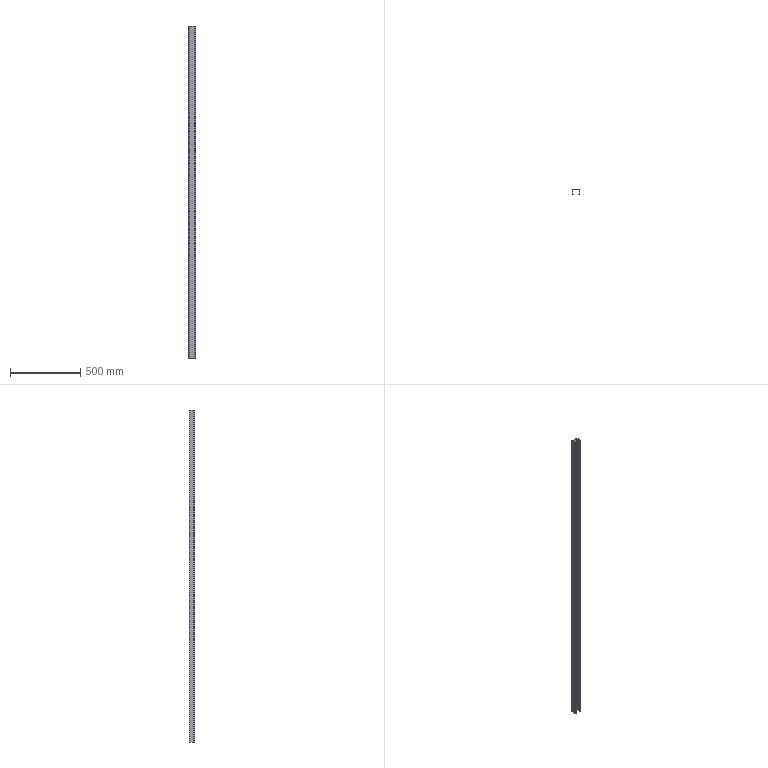Part | STEP file | 31E-01025QY25 | 1 solid | 28 faces | box 50 x 38.192 x 2366 mm | volume 389538 mm3 | plane 16 | cylinder 12 | commonest cylinder face diameters 1 x4 2 x4 4 x2 26 x2
STEP:
#1=CARTESIAN_POINT('',(27.993,8.298,1183.));
#2=VERTEX_POINT('',#1);
#3=CARTESIAN_POINT('',(32.281,3.187,1183.));
#4=VERTEX_POINT('',#3);
#5=CARTESIAN_POINT('',(30.137,5.743,1183.));
#6=DIRECTION('',(0.6428,-0.766,0.));
#7=VECTOR('',#6,1.);
#8=LINE('',#5,#7);
#9=EDGE_CURVE('',#2,#4,#8,.T.);
#10=ORIENTED_EDGE('',*,*,#9,.F.);
#11=CARTESIAN_POINT('',(27.993,8.298,-1183.));
#12=VERTEX_POINT('',#11);
#13=CARTESIAN_POINT('',(27.993,8.298,0.));
#14=DIRECTION('',(0.,0.,-1.));
#15=VECTOR('',#14,1.);
#16=LINE('',#13,#15);
#17=EDGE_CURVE('',#2,#12,#16,.T.);
#18=ORIENTED_EDGE('',*,*,#17,.T.);
#19=CARTESIAN_POINT('',(32.281,3.187,-1183.));
#20=VERTEX_POINT('',#19);
#21=CARTESIAN_POINT('',(30.137,5.743,-1183.));
#22=DIRECTION('',(0.6428,-0.766,0.));
#23=VECTOR('',#22,1.);
#24=LINE('',#21,#23);
#25=EDGE_CURVE('',#12,#20,#24,.T.);
#26=ORIENTED_EDGE('',*,*,#25,.T.);
#27=CARTESIAN_POINT('',(32.281,3.187,0.));
#28=DIRECTION('',(0.,0.,-1.));
#29=VECTOR('',#28,1.);
#30=LINE('',#27,#29);
#31=EDGE_CURVE('',#4,#20,#30,.T.);
#32=ORIENTED_EDGE('',*,*,#31,.F.);
#33=EDGE_LOOP('',(#10,#18,#26,#32));
#34=FACE_OUTER_BOUND('',#33,.T.);
#35=CARTESIAN_POINT('',(27.525,8.856,1183.));
#36=DIRECTION('',(0.766,0.6428,0.));
#37=DIRECTION('',(-0.6428,0.766,0.));
#38=AXIS2_PLACEMENT_3D('',#35,#36,#37);
#39=PLANE('',#38);
#40=ADVANCED_FACE('',(#34),#39,.F.);
#41=CARTESIAN_POINT('',(76.525,38.856,1183.));
#42=VERTEX_POINT('',#41);
#43=CARTESIAN_POINT('',(28.525,38.856,1183.));
#44=VERTEX_POINT('',#43);
#45=CARTESIAN_POINT('',(52.525,38.856,1183.));
#46=DIRECTION('',(-1.,0.,0.));
#47=VECTOR('',#46,1.);
#48=LINE('',#45,#47);
#49=EDGE_CURVE('',#42,#44,#48,.T.);
#50=ORIENTED_EDGE('',*,*,#49,.T.);
#51=CARTESIAN_POINT('',(27.525,37.856,1183.));
#52=VERTEX_POINT('',#51);
#53=CARTESIAN_POINT('',(28.525,37.856,1183.));
#54=DIRECTION('',(0.,0.,1.));
#55=AXIS2_PLACEMENT_3D('',#53,#54,$);
#56=CIRCLE('',#55,1.);
#57=EDGE_CURVE('',#44,#52,#56,.T.);
#58=ORIENTED_EDGE('',*,*,#57,.T.);
#59=CARTESIAN_POINT('',(27.525,9.584,1183.));
#60=VERTEX_POINT('',#59);
#61=CARTESIAN_POINT('',(27.525,23.72,1183.));
#62=DIRECTION('',(0.,-1.,0.));
#63=VECTOR('',#62,1.);
#64=LINE('',#61,#63);
#65=EDGE_CURVE('',#52,#60,#64,.T.);
#66=ORIENTED_EDGE('',*,*,#65,.T.);
#67=CARTESIAN_POINT('',(29.525,9.584,1183.));
#68=DIRECTION('',(0.,0.,1.));
#69=AXIS2_PLACEMENT_3D('',#67,#68,$);
#70=CIRCLE('',#69,2.);
#71=EDGE_CURVE('',#60,#2,#70,.T.);
#72=ORIENTED_EDGE('',*,*,#71,.T.);
#73=ORIENTED_EDGE('',*,*,#9,.T.);
#74=CARTESIAN_POINT('',(28.342,2.493,1183.));
#75=VERTEX_POINT('',#74);
#76=CARTESIAN_POINT('',(30.312,2.84,1183.));
#77=DIRECTION('',(-0.9848,-0.1736,0.));
#78=VECTOR('',#77,1.);
#79=LINE('',#76,#78);
#80=EDGE_CURVE('',#4,#75,#79,.T.);
#81=ORIENTED_EDGE('',*,*,#80,.T.);
#82=CARTESIAN_POINT('',(32.653,0.6877,1183.));
#83=VERTEX_POINT('',#82);
#84=CARTESIAN_POINT('',(35.437,13.386,1183.));
#85=DIRECTION('',(0.,0.,1.));
#86=AXIS2_PLACEMENT_3D('',#84,#85,$);
#87=CIRCLE('',#86,13.);
#88=EDGE_CURVE('',#75,#83,#87,.T.);
#89=ORIENTED_EDGE('',*,*,#88,.T.);
#90=CARTESIAN_POINT('',(33.867,1.665,1183.));
#91=VERTEX_POINT('',#90);
#92=CARTESIAN_POINT('',(32.867,1.665,1183.));
#93=DIRECTION('',(0.,0.,1.));
#94=AXIS2_PLACEMENT_3D('',#92,#93,$);
#95=CIRCLE('',#94,1.);
#96=EDGE_CURVE('',#83,#91,#95,.T.);
#97=ORIENTED_EDGE('',*,*,#96,.T.);
#98=CARTESIAN_POINT('',(33.867,2.983,1183.));
#99=VERTEX_POINT('',#98);
#100=CARTESIAN_POINT('',(33.867,2.324,1183.));
#101=DIRECTION('',(0.,1.,0.));
#102=VECTOR('',#101,1.);
#103=LINE('',#100,#102);
#104=EDGE_CURVE('',#91,#99,#103,.T.);
#105=ORIENTED_EDGE('',*,*,#104,.T.);
#106=CARTESIAN_POINT('',(33.75,3.304,1183.));
#107=VERTEX_POINT('',#106);
#108=CARTESIAN_POINT('',(33.367,2.983,1183.));
#109=DIRECTION('',(0.,0.,1.));
#110=AXIS2_PLACEMENT_3D('',#108,#109,$);
#111=CIRCLE('',#110,0.5);
#112=EDGE_CURVE('',#99,#107,#111,.T.);
#113=ORIENTED_EDGE('',*,*,#112,.T.);
#114=CARTESIAN_POINT('',(28.725,9.293,1183.));
#115=VERTEX_POINT('',#114);
#116=CARTESIAN_POINT('',(31.237,6.298,1183.));
#117=DIRECTION('',(-0.6428,0.766,0.));
#118=VECTOR('',#117,1.);
#119=LINE('',#116,#118);
#120=EDGE_CURVE('',#107,#115,#119,.T.);
#121=ORIENTED_EDGE('',*,*,#120,.T.);
#122=CARTESIAN_POINT('',(28.725,37.156,1183.));
#123=VERTEX_POINT('',#122);
#124=CARTESIAN_POINT('',(28.725,23.225,1183.));
#125=DIRECTION('',(0.,1.,0.));
#126=VECTOR('',#125,1.);
#127=LINE('',#124,#126);
#128=EDGE_CURVE('',#115,#123,#127,.T.);
#129=ORIENTED_EDGE('',*,*,#128,.T.);
#130=CARTESIAN_POINT('',(29.225,37.656,1183.));
#131=VERTEX_POINT('',#130);
#132=CARTESIAN_POINT('',(28.725,37.156,1183.));
#133=CARTESIAN_POINT('',(28.725,37.219,1183.));
#134=CARTESIAN_POINT('',(28.735,37.282,1183.));
#135=CARTESIAN_POINT('',(28.754,37.343,1183.));
#136=CARTESIAN_POINT('',(28.812,37.456,1183.));
#137=CARTESIAN_POINT('',(28.902,37.546,1183.));
#138=CARTESIAN_POINT('',(28.954,37.583,1183.));
#139=CARTESIAN_POINT('',(29.039,37.627,1183.));
#140=CARTESIAN_POINT('',(29.131,37.649,1183.));
#141=CARTESIAN_POINT('',(29.162,37.654,1183.));
#142=CARTESIAN_POINT('',(29.193,37.656,1183.));
#143=CARTESIAN_POINT('',(29.225,37.656,1183.));
#144=B_SPLINE_CURVE_WITH_KNOTS('',5,(#132,#133,#134,#135,#136,#137,#138,#139,#140,#141,#142,#143),.UNSPECIFIED.,.F.,.U.,(6,3,3,6),(0.,0.4443,0.8886,1.11),.UNSPECIFIED.);
#145=EDGE_CURVE('',#123,#131,#144,.T.);
#146=ORIENTED_EDGE('',*,*,#145,.T.);
#147=CARTESIAN_POINT('',(75.825,37.656,1183.));
#148=VERTEX_POINT('',#147);
#149=CARTESIAN_POINT('',(52.525,37.656,1183.));
#150=DIRECTION('',(1.,0.,0.));
#151=VECTOR('',#150,1.);
#152=LINE('',#149,#151);
#153=EDGE_CURVE('',#131,#148,#152,.T.);
#154=ORIENTED_EDGE('',*,*,#153,.T.);
#155=CARTESIAN_POINT('',(76.325,37.156,1183.));
#156=VERTEX_POINT('',#155);
#157=CARTESIAN_POINT('',(75.825,37.656,1183.));
#158=CARTESIAN_POINT('',(75.888,37.656,1183.));
#159=CARTESIAN_POINT('',(75.95,37.646,1183.));
#160=CARTESIAN_POINT('',(76.011,37.627,1183.));
#161=CARTESIAN_POINT('',(76.124,37.569,1183.));
#162=CARTESIAN_POINT('',(76.214,37.479,1183.));
#163=CARTESIAN_POINT('',(76.252,37.427,1183.));
#164=CARTESIAN_POINT('',(76.295,37.342,1183.));
#165=CARTESIAN_POINT('',(76.317,37.25,1183.));
#166=CARTESIAN_POINT('',(76.322,37.219,1183.));
#167=CARTESIAN_POINT('',(76.325,37.187,1183.));
#168=CARTESIAN_POINT('',(76.325,37.156,1183.));
#169=B_SPLINE_CURVE_WITH_KNOTS('',5,(#157,#158,#159,#160,#161,#162,#163,#164,#165,#166,#167,#168),.UNSPECIFIED.,.F.,.U.,(6,3,3,6),(0.,0.4443,0.8886,1.11),.UNSPECIFIED.);
#170=EDGE_CURVE('',#148,#156,#169,.T.);
#171=ORIENTED_EDGE('',*,*,#170,.T.);
#172=CARTESIAN_POINT('',(76.325,9.293,1183.));
#173=VERTEX_POINT('',#172);
#174=CARTESIAN_POINT('',(76.325,23.225,1183.));
#175=DIRECTION('',(0.,-1.,0.));
#176=VECTOR('',#175,1.);
#177=LINE('',#174,#176);
#178=EDGE_CURVE('',#156,#173,#177,.T.);
#179=ORIENTED_EDGE('',*,*,#178,.T.);
#180=CARTESIAN_POINT('',(71.299,3.304,1183.));
#181=VERTEX_POINT('',#180);
#182=CARTESIAN_POINT('',(73.812,6.298,1183.));
#183=DIRECTION('',(-0.6428,-0.766,0.));
#184=VECTOR('',#183,1.);
#185=LINE('',#182,#184);
#186=EDGE_CURVE('',#173,#181,#185,.T.);
#187=ORIENTED_EDGE('',*,*,#186,.T.);
#188=CARTESIAN_POINT('',(71.182,2.983,1183.));
#189=VERTEX_POINT('',#188);
#190=CARTESIAN_POINT('',(71.682,2.983,1183.));
#191=DIRECTION('',(0.,0.,1.));
#192=AXIS2_PLACEMENT_3D('',#190,#191,$);
#193=CIRCLE('',#192,0.5);
#194=EDGE_CURVE('',#181,#189,#193,.T.);
#195=ORIENTED_EDGE('',*,*,#194,.T.);
#196=CARTESIAN_POINT('',(71.182,1.665,1183.));
#197=VERTEX_POINT('',#196);
#198=CARTESIAN_POINT('',(71.182,2.324,1183.));
#199=DIRECTION('',(0.,-1.,0.));
#200=VECTOR('',#199,1.);
#201=LINE('',#198,#200);
#202=EDGE_CURVE('',#189,#197,#201,.T.);
#203=ORIENTED_EDGE('',*,*,#202,.T.);
#204=CARTESIAN_POINT('',(72.397,0.6877,1183.));
#205=VERTEX_POINT('',#204);
#206=CARTESIAN_POINT('',(72.182,1.665,1183.));
#207=DIRECTION('',(0.,0.,1.));
#208=AXIS2_PLACEMENT_3D('',#206,#207,$);
#209=CIRCLE('',#208,1.);
#210=EDGE_CURVE('',#197,#205,#209,.T.);
#211=ORIENTED_EDGE('',*,*,#210,.T.);
#212=CARTESIAN_POINT('',(76.707,2.493,1183.));
#213=VERTEX_POINT('',#212);
#214=CARTESIAN_POINT('',(69.613,13.386,1183.));
#215=DIRECTION('',(0.,0.,1.));
#216=AXIS2_PLACEMENT_3D('',#214,#215,$);
#217=CIRCLE('',#216,13.);
#218=EDGE_CURVE('',#205,#213,#217,.T.);
#219=ORIENTED_EDGE('',*,*,#218,.T.);
#220=CARTESIAN_POINT('',(72.768,3.187,1183.));
#221=VERTEX_POINT('',#220);
#222=CARTESIAN_POINT('',(74.738,2.84,1183.));
#223=DIRECTION('',(-0.9848,0.1736,0.));
#224=VECTOR('',#223,1.);
#225=LINE('',#222,#224);
#226=EDGE_CURVE('',#213,#221,#225,.T.);
#227=ORIENTED_EDGE('',*,*,#226,.T.);
#228=CARTESIAN_POINT('',(77.057,8.298,1183.));
#229=VERTEX_POINT('',#228);
#230=CARTESIAN_POINT('',(74.912,5.743,1183.));
#231=DIRECTION('',(0.6428,0.766,0.));
#232=VECTOR('',#231,1.);
#233=LINE('',#230,#232);
#234=EDGE_CURVE('',#221,#229,#233,.T.);
#235=ORIENTED_EDGE('',*,*,#234,.T.);
#236=CARTESIAN_POINT('',(77.525,9.584,1183.));
#237=VERTEX_POINT('',#236);
#238=CARTESIAN_POINT('',(75.525,9.584,1183.));
#239=DIRECTION('',(0.,0.,1.));
#240=AXIS2_PLACEMENT_3D('',#238,#239,$);
#241=CIRCLE('',#240,2.);
#242=EDGE_CURVE('',#229,#237,#241,.T.);
#243=ORIENTED_EDGE('',*,*,#242,.T.);
#244=CARTESIAN_POINT('',(77.525,37.856,1183.));
#245=VERTEX_POINT('',#244);
#246=CARTESIAN_POINT('',(77.525,23.72,1183.));
#247=DIRECTION('',(0.,1.,0.));
#248=VECTOR('',#247,1.);
#249=LINE('',#246,#248);
#250=EDGE_CURVE('',#237,#245,#249,.T.);
#251=ORIENTED_EDGE('',*,*,#250,.T.);
#252=CARTESIAN_POINT('',(76.525,37.856,1183.));
#253=DIRECTION('',(0.,0.,1.));
#254=AXIS2_PLACEMENT_3D('',#252,#253,$);
#255=CIRCLE('',#254,1.);
#256=EDGE_CURVE('',#245,#42,#255,.T.);
#257=ORIENTED_EDGE('',*,*,#256,.T.);
#258=EDGE_LOOP('',(#50,#58,#66,#72,#73,#81,#89,#97,#105,#113,#121,#129,#146,#154,#171,#179,#187,#195,#203,#211,#219,#227,#235,#243,#251,#257));
#259=FACE_OUTER_BOUND('',#258,.T.);
#260=CARTESIAN_POINT('',(35.437,13.386,1183.));
#261=DIRECTION('',(0.,0.,1.));
#262=DIRECTION('',(1.,0.,0.));
#263=AXIS2_PLACEMENT_3D('',#260,#261,#262);
#264=PLANE('',#263);
#265=ADVANCED_FACE('',(#259),#264,.T.);
#266=ORIENTED_EDGE('',*,*,#71,.F.);
#267=CARTESIAN_POINT('',(27.525,9.584,-1183.));
#268=VERTEX_POINT('',#267);
#269=CARTESIAN_POINT('',(27.525,9.584,1183.));
#270=DIRECTION('',(0.,0.,-1.));
#271=VECTOR('',#270,1.);
#272=LINE('',#269,#271);
#273=EDGE_CURVE('',#268,#60,#272,.F.);
#274=ORIENTED_EDGE('',*,*,#273,.F.);
#275=CARTESIAN_POINT('',(29.525,9.584,-1183.));
#276=DIRECTION('',(0.,0.,-1.));
#277=AXIS2_PLACEMENT_3D('',#275,#276,$);
#278=CIRCLE('',#277,2.);
#279=EDGE_CURVE('',#12,#268,#278,.T.);
#280=ORIENTED_EDGE('',*,*,#279,.F.);
#281=ORIENTED_EDGE('',*,*,#17,.F.);
#282=EDGE_LOOP('',(#266,#274,#280,#281));
#283=FACE_OUTER_BOUND('',#282,.T.);
#284=CARTESIAN_POINT('',(29.525,9.584,1183.));
#285=DIRECTION('',(0.,0.,-1.));
#286=DIRECTION('',(1.,0.,0.));
#287=AXIS2_PLACEMENT_3D('',#284,#285,#286);
#288=CYLINDRICAL_SURFACE('',#287,2.);
#289=ADVANCED_FACE('',(#283),#288,.T.);
#290=CARTESIAN_POINT('',(27.525,37.856,-1183.));
#291=VERTEX_POINT('',#290);
#292=CARTESIAN_POINT('',(28.525,38.856,-1183.));
#293=VERTEX_POINT('',#292);
#294=CARTESIAN_POINT('',(27.525,37.856,-1183.));
#295=CARTESIAN_POINT('',(27.525,37.954,-1183.));
#296=CARTESIAN_POINT('',(27.537,38.052,-1183.));
#297=CARTESIAN_POINT('',(27.561,38.148,-1183.));
#298=CARTESIAN_POINT('',(27.632,38.332,-1183.));
#299=CARTESIAN_POINT('',(27.745,38.494,-1183.));
#300=CARTESIAN_POINT('',(27.812,38.567,-1183.));
#301=CARTESIAN_POINT('',(27.961,38.696,-1183.));
#302=CARTESIAN_POINT('',(28.137,38.786,-1183.));
#303=CARTESIAN_POINT('',(28.23,38.819,-1183.));
#304=CARTESIAN_POINT('',(28.346,38.846,-1183.));
#305=CARTESIAN_POINT('',(28.464,38.855,-1183.));
#306=CARTESIAN_POINT('',(28.484,38.856,-1183.));
#307=CARTESIAN_POINT('',(28.505,38.856,-1183.));
#308=CARTESIAN_POINT('',(28.525,38.856,-1183.));
#309=B_SPLINE_CURVE_WITH_KNOTS('',5,(#294,#295,#296,#297,#298,#299,#300,#301,#302,#303,#304,#305,#306,#307,#308),.UNSPECIFIED.,.F.,.U.,(6,3,3,3,6),(0.,0.6928,1.386,2.078,2.221),.UNSPECIFIED.);
#310=EDGE_CURVE('',#291,#293,#309,.T.);
#311=ORIENTED_EDGE('',*,*,#310,.T.);
#312=CARTESIAN_POINT('',(76.525,38.856,-1183.));
#313=VERTEX_POINT('',#312);
#314=CARTESIAN_POINT('',(52.525,38.856,-1183.));
#315=DIRECTION('',(-1.,0.,0.));
#316=VECTOR('',#315,1.);
#317=LINE('',#314,#316);
#318=EDGE_CURVE('',#313,#293,#317,.T.);
#319=ORIENTED_EDGE('',*,*,#318,.F.);
#320=CARTESIAN_POINT('',(77.525,37.856,-1183.));
#321=VERTEX_POINT('',#320);
#322=CARTESIAN_POINT('',(76.525,38.856,-1183.));
#323=CARTESIAN_POINT('',(76.623,38.856,-1183.));
#324=CARTESIAN_POINT('',(76.721,38.844,-1183.));
#325=CARTESIAN_POINT('',(76.817,38.82,-1183.));
#326=CARTESIAN_POINT('',(77.001,38.749,-1183.));
#327=CARTESIAN_POINT('',(77.163,38.636,-1183.));
#328=CARTESIAN_POINT('',(77.236,38.569,-1183.));
#329=CARTESIAN_POINT('',(77.365,38.42,-1183.));
#330=CARTESIAN_POINT('',(77.454,38.244,-1183.));
#331=CARTESIAN_POINT('',(77.488,38.151,-1183.));
#332=CARTESIAN_POINT('',(77.514,38.035,-1183.));
#333=CARTESIAN_POINT('',(77.523,37.917,-1183.));
#334=CARTESIAN_POINT('',(77.524,37.897,-1183.));
#335=CARTESIAN_POINT('',(77.525,37.876,-1183.));
#336=CARTESIAN_POINT('',(77.525,37.856,-1183.));
#337=B_SPLINE_CURVE_WITH_KNOTS('',5,(#322,#323,#324,#325,#326,#327,#328,#329,#330,#331,#332,#333,#334,#335,#336),.UNSPECIFIED.,.F.,.U.,(6,3,3,3,6),(0.,0.6928,1.386,2.078,2.221),.UNSPECIFIED.);
#338=EDGE_CURVE('',#313,#321,#337,.T.);
#339=ORIENTED_EDGE('',*,*,#338,.T.);
#340=CARTESIAN_POINT('',(77.525,9.584,-1183.));
#341=VERTEX_POINT('',#340);
#342=CARTESIAN_POINT('',(77.525,23.72,-1183.));
#343=DIRECTION('',(0.,1.,0.));
#344=VECTOR('',#343,1.);
#345=LINE('',#342,#344);
#346=EDGE_CURVE('',#341,#321,#345,.T.);
#347=ORIENTED_EDGE('',*,*,#346,.F.);
#348=CARTESIAN_POINT('',(77.057,8.298,-1183.));
#349=VERTEX_POINT('',#348);
#350=CARTESIAN_POINT('',(77.525,9.584,-1183.));
#351=CARTESIAN_POINT('',(77.525,9.361,-1183.));
#352=CARTESIAN_POINT('',(77.494,9.137,-1183.));
#353=CARTESIAN_POINT('',(77.431,8.92,-1183.));
#354=CARTESIAN_POINT('',(77.316,8.662,-1183.));
#355=CARTESIAN_POINT('',(77.16,8.431,-1183.));
#356=CARTESIAN_POINT('',(77.127,8.385,-1183.));
#357=CARTESIAN_POINT('',(77.093,8.341,-1183.));
#358=CARTESIAN_POINT('',(77.057,8.298,-1183.));
#359=B_SPLINE_CURVE_WITH_KNOTS('',5,(#350,#351,#352,#353,#354,#355,#356,#357,#358),.UNSPECIFIED.,.F.,.U.,(6,3,6),(0.,1.58,1.974),.UNSPECIFIED.);
#360=EDGE_CURVE('',#341,#349,#359,.T.);
#361=ORIENTED_EDGE('',*,*,#360,.T.);
#362=CARTESIAN_POINT('',(72.768,3.187,-1183.));
#363=VERTEX_POINT('',#362);
#364=CARTESIAN_POINT('',(74.912,5.743,-1183.));
#365=DIRECTION('',(0.6428,0.766,0.));
#366=VECTOR('',#365,1.);
#367=LINE('',#364,#366);
#368=EDGE_CURVE('',#363,#349,#367,.T.);
#369=ORIENTED_EDGE('',*,*,#368,.F.);
#370=CARTESIAN_POINT('',(76.707,2.493,-1183.));
#371=VERTEX_POINT('',#370);
#372=CARTESIAN_POINT('',(74.738,2.84,-1183.));
#373=DIRECTION('',(-0.9848,0.1736,0.));
#374=VECTOR('',#373,1.);
#375=LINE('',#372,#374);
#376=EDGE_CURVE('',#371,#363,#375,.T.);
#377=ORIENTED_EDGE('',*,*,#376,.F.);
#378=CARTESIAN_POINT('',(72.397,0.6877,-1183.));
#379=VERTEX_POINT('',#378);
#380=CARTESIAN_POINT('',(69.613,13.386,-1183.));
#381=DIRECTION('',(0.,0.,1.));
#382=AXIS2_PLACEMENT_3D('',#380,#381,$);
#383=CIRCLE('',#382,13.);
#384=EDGE_CURVE('',#379,#371,#383,.T.);
#385=ORIENTED_EDGE('',*,*,#384,.F.);
#386=CARTESIAN_POINT('',(71.182,1.665,-1183.));
#387=VERTEX_POINT('',#386);
#388=CARTESIAN_POINT('',(72.182,1.665,-1183.));
#389=DIRECTION('',(0.,0.,1.));
#390=AXIS2_PLACEMENT_3D('',#388,#389,$);
#391=CIRCLE('',#390,1.);
#392=EDGE_CURVE('',#387,#379,#391,.T.);
#393=ORIENTED_EDGE('',*,*,#392,.F.);
#394=CARTESIAN_POINT('',(71.182,2.983,-1183.));
#395=VERTEX_POINT('',#394);
#396=CARTESIAN_POINT('',(71.182,2.324,-1183.));
#397=DIRECTION('',(0.,-1.,0.));
#398=VECTOR('',#397,1.);
#399=LINE('',#396,#398);
#400=EDGE_CURVE('',#395,#387,#399,.T.);
#401=ORIENTED_EDGE('',*,*,#400,.F.);
#402=CARTESIAN_POINT('',(71.299,3.304,-1183.));
#403=VERTEX_POINT('',#402);
#404=CARTESIAN_POINT('',(71.182,2.983,-1183.));
#405=CARTESIAN_POINT('',(71.182,3.038,-1183.));
#406=CARTESIAN_POINT('',(71.19,3.094,-1183.));
#407=CARTESIAN_POINT('',(71.206,3.149,-1183.));
#408=CARTESIAN_POINT('',(71.235,3.213,-1183.));
#409=CARTESIAN_POINT('',(71.274,3.271,-1183.));
#410=CARTESIAN_POINT('',(71.282,3.282,-1183.));
#411=CARTESIAN_POINT('',(71.29,3.293,-1183.));
#412=CARTESIAN_POINT('',(71.299,3.304,-1183.));
#413=B_SPLINE_CURVE_WITH_KNOTS('',5,(#404,#405,#406,#407,#408,#409,#410,#411,#412),.UNSPECIFIED.,.F.,.U.,(6,3,6),(0.,0.3949,0.4936),.UNSPECIFIED.);
#414=EDGE_CURVE('',#395,#403,#413,.T.);
#415=ORIENTED_EDGE('',*,*,#414,.T.);
#416=CARTESIAN_POINT('',(76.325,9.293,-1183.));
#417=VERTEX_POINT('',#416);
#418=CARTESIAN_POINT('',(73.812,6.298,-1183.));
#419=DIRECTION('',(-0.6428,-0.766,0.));
#420=VECTOR('',#419,1.);
#421=LINE('',#418,#420);
#422=EDGE_CURVE('',#417,#403,#421,.T.);
#423=ORIENTED_EDGE('',*,*,#422,.F.);
#424=CARTESIAN_POINT('',(76.325,37.156,-1183.));
#425=VERTEX_POINT('',#424);
#426=CARTESIAN_POINT('',(76.325,23.225,-1183.));
#427=DIRECTION('',(0.,-1.,0.));
#428=VECTOR('',#427,1.);
#429=LINE('',#426,#428);
#430=EDGE_CURVE('',#425,#417,#429,.T.);
#431=ORIENTED_EDGE('',*,*,#430,.F.);
#432=CARTESIAN_POINT('',(75.825,37.656,-1183.));
#433=VERTEX_POINT('',#432);
#434=CARTESIAN_POINT('',(75.825,37.156,-1183.));
#435=DIRECTION('',(0.,0.,1.));
#436=AXIS2_PLACEMENT_3D('',#434,#435,$);
#437=CIRCLE('',#436,0.5);
#438=EDGE_CURVE('',#425,#433,#437,.T.);
#439=ORIENTED_EDGE('',*,*,#438,.T.);
#440=CARTESIAN_POINT('',(29.225,37.656,-1183.));
#441=VERTEX_POINT('',#440);
#442=CARTESIAN_POINT('',(52.525,37.656,-1183.));
#443=DIRECTION('',(1.,0.,0.));
#444=VECTOR('',#443,1.);
#445=LINE('',#442,#444);
#446=EDGE_CURVE('',#441,#433,#445,.T.);
#447=ORIENTED_EDGE('',*,*,#446,.F.);
#448=CARTESIAN_POINT('',(28.725,37.156,-1183.));
#449=VERTEX_POINT('',#448);
#450=CARTESIAN_POINT('',(29.225,37.156,-1183.));
#451=DIRECTION('',(0.,0.,1.));
#452=AXIS2_PLACEMENT_3D('',#450,#451,$);
#453=CIRCLE('',#452,0.5);
#454=EDGE_CURVE('',#441,#449,#453,.T.);
#455=ORIENTED_EDGE('',*,*,#454,.T.);
#456=CARTESIAN_POINT('',(28.725,9.293,-1183.));
#457=VERTEX_POINT('',#456);
#458=CARTESIAN_POINT('',(28.725,23.225,-1183.));
#459=DIRECTION('',(0.,1.,0.));
#460=VECTOR('',#459,1.);
#461=LINE('',#458,#460);
#462=EDGE_CURVE('',#457,#449,#461,.T.);
#463=ORIENTED_EDGE('',*,*,#462,.F.);
#464=CARTESIAN_POINT('',(33.75,3.304,-1183.));
#465=VERTEX_POINT('',#464);
#466=CARTESIAN_POINT('',(31.237,6.298,-1183.));
#467=DIRECTION('',(-0.6428,0.766,0.));
#468=VECTOR('',#467,1.);
#469=LINE('',#466,#468);
#470=EDGE_CURVE('',#465,#457,#469,.T.);
#471=ORIENTED_EDGE('',*,*,#470,.F.);
#472=CARTESIAN_POINT('',(33.867,2.983,-1183.));
#473=VERTEX_POINT('',#472);
#474=CARTESIAN_POINT('',(33.75,3.304,-1183.));
#475=CARTESIAN_POINT('',(33.786,3.261,-1183.));
#476=CARTESIAN_POINT('',(33.816,3.213,-1183.));
#477=CARTESIAN_POINT('',(33.839,3.162,-1183.));
#478=CARTESIAN_POINT('',(33.858,3.094,-1183.));
#479=CARTESIAN_POINT('',(33.866,3.024,-1183.));
#480=CARTESIAN_POINT('',(33.867,3.01,-1183.));
#481=CARTESIAN_POINT('',(33.867,2.997,-1183.));
#482=CARTESIAN_POINT('',(33.867,2.983,-1183.));
#483=B_SPLINE_CURVE_WITH_KNOTS('',5,(#474,#475,#476,#477,#478,#479,#480,#481,#482),.UNSPECIFIED.,.F.,.U.,(6,3,6),(0.,0.3949,0.4936),.UNSPECIFIED.);
#484=EDGE_CURVE('',#465,#473,#483,.T.);
#485=ORIENTED_EDGE('',*,*,#484,.T.);
#486=CARTESIAN_POINT('',(33.867,1.665,-1183.));
#487=VERTEX_POINT('',#486);
#488=CARTESIAN_POINT('',(33.867,2.324,-1183.));
#489=DIRECTION('',(0.,1.,0.));
#490=VECTOR('',#489,1.);
#491=LINE('',#488,#490);
#492=EDGE_CURVE('',#487,#473,#491,.T.);
#493=ORIENTED_EDGE('',*,*,#492,.F.);
#494=CARTESIAN_POINT('',(32.653,0.6877,-1183.));
#495=VERTEX_POINT('',#494);
#496=CARTESIAN_POINT('',(32.867,1.665,-1183.));
#497=DIRECTION('',(0.,0.,1.));
#498=AXIS2_PLACEMENT_3D('',#496,#497,$);
#499=CIRCLE('',#498,1.);
#500=EDGE_CURVE('',#495,#487,#499,.T.);
#501=ORIENTED_EDGE('',*,*,#500,.F.);
#502=CARTESIAN_POINT('',(28.342,2.493,-1183.));
#503=VERTEX_POINT('',#502);
#504=CARTESIAN_POINT('',(35.437,13.386,-1183.));
#505=DIRECTION('',(0.,0.,1.));
#506=AXIS2_PLACEMENT_3D('',#504,#505,$);
#507=CIRCLE('',#506,13.);
#508=EDGE_CURVE('',#503,#495,#507,.T.);
#509=ORIENTED_EDGE('',*,*,#508,.F.);
#510=CARTESIAN_POINT('',(30.312,2.84,-1183.));
#511=DIRECTION('',(-0.9848,-0.1736,0.));
#512=VECTOR('',#511,1.);
#513=LINE('',#510,#512);
#514=EDGE_CURVE('',#20,#503,#513,.T.);
#515=ORIENTED_EDGE('',*,*,#514,.F.);
#516=ORIENTED_EDGE('',*,*,#25,.F.);
#517=ORIENTED_EDGE('',*,*,#279,.T.);
#518=CARTESIAN_POINT('',(27.525,23.72,-1183.));
#519=DIRECTION('',(0.,-1.,0.));
#520=VECTOR('',#519,1.);
#521=LINE('',#518,#520);
#522=EDGE_CURVE('',#291,#268,#521,.T.);
#523=ORIENTED_EDGE('',*,*,#522,.F.);
#524=EDGE_LOOP('',(#311,#319,#339,#347,#361,#369,#377,#385,#393,#401,#415,#423,#431,#439,#447,#455,#463,#471,#485,#493,#501,#509,#515,#516,#517,#523));
#525=FACE_OUTER_BOUND('',#524,.T.);
#526=CARTESIAN_POINT('',(35.437,13.386,-1183.));
#527=DIRECTION('',(0.,0.,1.));
#528=DIRECTION('',(1.,0.,0.));
#529=AXIS2_PLACEMENT_3D('',#526,#527,#528);
#530=PLANE('',#529);
#531=ADVANCED_FACE('',(#525),#530,.F.);
#532=ORIENTED_EDGE('',*,*,#514,.T.);
#533=CARTESIAN_POINT('',(28.342,2.493,0.));
#534=DIRECTION('',(0.,0.,-1.));
#535=VECTOR('',#534,1.);
#536=LINE('',#533,#535);
#537=EDGE_CURVE('',#75,#503,#536,.T.);
#538=ORIENTED_EDGE('',*,*,#537,.F.);
#539=ORIENTED_EDGE('',*,*,#80,.F.);
#540=ORIENTED_EDGE('',*,*,#31,.T.);
#541=EDGE_LOOP('',(#532,#538,#539,#540));
#542=FACE_OUTER_BOUND('',#541,.T.);
#543=CARTESIAN_POINT('',(32.281,3.187,1183.));
#544=DIRECTION('',(0.1736,-0.9848,0.));
#545=DIRECTION('',(0.9848,0.1736,0.));
#546=AXIS2_PLACEMENT_3D('',#543,#544,#545);
#547=PLANE('',#546);
#548=ADVANCED_FACE('',(#542),#547,.F.);
#549=ORIENTED_EDGE('',*,*,#318,.T.);
#550=CARTESIAN_POINT('',(28.525,38.856,0.));
#551=DIRECTION('',(0.,0.,1.));
#552=VECTOR('',#551,1.);
#553=LINE('',#550,#552);
#554=EDGE_CURVE('',#293,#44,#553,.T.);
#555=ORIENTED_EDGE('',*,*,#554,.T.);
#556=ORIENTED_EDGE('',*,*,#49,.F.);
#557=CARTESIAN_POINT('',(76.525,38.856,0.));
#558=DIRECTION('',(0.,0.,-1.));
#559=VECTOR('',#558,1.);
#560=LINE('',#557,#559);
#561=EDGE_CURVE('',#42,#313,#560,.T.);
#562=ORIENTED_EDGE('',*,*,#561,.T.);
#563=EDGE_LOOP('',(#549,#555,#556,#562));
#564=FACE_OUTER_BOUND('',#563,.T.);
#565=CARTESIAN_POINT('',(27.525,38.856,1183.));
#566=DIRECTION('',(0.,-1.,0.));
#567=DIRECTION('',(1.,0.,0.));
#568=AXIS2_PLACEMENT_3D('',#565,#566,#567);
#569=PLANE('',#568);
#570=ADVANCED_FACE('',(#564),#569,.F.);
#571=ORIENTED_EDGE('',*,*,#57,.F.);
#572=ORIENTED_EDGE('',*,*,#554,.F.);
#573=ORIENTED_EDGE('',*,*,#310,.F.);
#574=CARTESIAN_POINT('',(27.525,37.856,1183.));
#575=DIRECTION('',(0.,0.,-1.));
#576=VECTOR('',#575,1.);
#577=LINE('',#574,#576);
#578=EDGE_CURVE('',#52,#291,#577,.T.);
#579=ORIENTED_EDGE('',*,*,#578,.F.);
#580=EDGE_LOOP('',(#571,#572,#573,#579));
#581=FACE_OUTER_BOUND('',#580,.T.);
#582=CARTESIAN_POINT('',(28.525,37.856,1183.));
#583=DIRECTION('',(0.,0.,-1.));
#584=DIRECTION('',(-1.,0.,0.));
#585=AXIS2_PLACEMENT_3D('',#582,#583,#584);
#586=CYLINDRICAL_SURFACE('',#585,1.);
#587=ADVANCED_FACE('',(#581),#586,.T.);
#588=ORIENTED_EDGE('',*,*,#65,.F.);
#589=ORIENTED_EDGE('',*,*,#578,.T.);
#590=ORIENTED_EDGE('',*,*,#522,.T.);
#591=ORIENTED_EDGE('',*,*,#273,.T.);
#592=EDGE_LOOP('',(#588,#589,#590,#591));
#593=FACE_OUTER_BOUND('',#592,.T.);
#594=CARTESIAN_POINT('',(27.525,8.856,1183.));
#595=DIRECTION('',(1.,0.,0.));
#596=DIRECTION('',(0.,0.,-1.));
#597=AXIS2_PLACEMENT_3D('',#594,#595,#596);
#598=PLANE('',#597);
#599=ADVANCED_FACE('',(#593),#598,.F.);
#600=ORIENTED_EDGE('',*,*,#508,.T.);
#601=CARTESIAN_POINT('',(32.653,0.6877,1183.));
#602=DIRECTION('',(0.,0.,-1.));
#603=VECTOR('',#602,1.);
#604=LINE('',#601,#603);
#605=EDGE_CURVE('',#83,#495,#604,.T.);
#606=ORIENTED_EDGE('',*,*,#605,.F.);
#607=ORIENTED_EDGE('',*,*,#88,.F.);
#608=ORIENTED_EDGE('',*,*,#537,.T.);
#609=EDGE_LOOP('',(#600,#606,#607,#608));
#610=FACE_OUTER_BOUND('',#609,.T.);
#611=CARTESIAN_POINT('',(35.437,13.386,1183.));
#612=DIRECTION('',(0.,0.,-1.));
#613=DIRECTION('',(1.,0.,0.));
#614=AXIS2_PLACEMENT_3D('',#611,#612,#613);
#615=CYLINDRICAL_SURFACE('',#614,13.);
#616=ADVANCED_FACE('',(#610),#615,.T.);
#617=ORIENTED_EDGE('',*,*,#500,.T.);
#618=CARTESIAN_POINT('',(33.867,1.665,1183.));
#619=DIRECTION('',(0.,0.,-1.));
#620=VECTOR('',#619,1.);
#621=LINE('',#618,#620);
#622=EDGE_CURVE('',#91,#487,#621,.T.);
#623=ORIENTED_EDGE('',*,*,#622,.F.);
#624=ORIENTED_EDGE('',*,*,#96,.F.);
#625=ORIENTED_EDGE('',*,*,#605,.T.);
#626=EDGE_LOOP('',(#617,#623,#624,#625));
#627=FACE_OUTER_BOUND('',#626,.T.);
#628=CARTESIAN_POINT('',(32.867,1.665,1183.));
#629=DIRECTION('',(0.,0.,-1.));
#630=DIRECTION('',(1.,0.,0.));
#631=AXIS2_PLACEMENT_3D('',#628,#629,#630);
#632=CYLINDRICAL_SURFACE('',#631,1.);
#633=ADVANCED_FACE('',(#627),#632,.T.);
#634=ORIENTED_EDGE('',*,*,#492,.T.);
#635=CARTESIAN_POINT('',(33.867,2.983,0.));
#636=DIRECTION('',(0.,0.,1.));
#637=VECTOR('',#636,1.);
#638=LINE('',#635,#637);
#639=EDGE_CURVE('',#473,#99,#638,.T.);
#640=ORIENTED_EDGE('',*,*,#639,.T.);
#641=ORIENTED_EDGE('',*,*,#104,.F.);
#642=ORIENTED_EDGE('',*,*,#622,.T.);
#643=EDGE_LOOP('',(#634,#640,#641,#642));
#644=FACE_OUTER_BOUND('',#643,.T.);
#645=CARTESIAN_POINT('',(33.867,1.665,1183.));
#646=DIRECTION('',(-1.,0.,0.));
#647=DIRECTION('',(0.,0.,1.));
#648=AXIS2_PLACEMENT_3D('',#645,#646,#647);
#649=PLANE('',#648);
#650=ADVANCED_FACE('',(#644),#649,.F.);
#651=ORIENTED_EDGE('',*,*,#112,.F.);
#652=ORIENTED_EDGE('',*,*,#639,.F.);
#653=ORIENTED_EDGE('',*,*,#484,.F.);
#654=CARTESIAN_POINT('',(33.75,3.304,1183.));
#655=DIRECTION('',(0.,0.,-1.));
#656=VECTOR('',#655,1.);
#657=LINE('',#654,#656);
#658=EDGE_CURVE('',#107,#465,#657,.T.);
#659=ORIENTED_EDGE('',*,*,#658,.F.);
#660=EDGE_LOOP('',(#651,#652,#653,#659));
#661=FACE_OUTER_BOUND('',#660,.T.);
#662=CARTESIAN_POINT('',(33.367,2.983,1183.));
#663=DIRECTION('',(0.,0.,-1.));
#664=DIRECTION('',(-1.,0.,0.));
#665=AXIS2_PLACEMENT_3D('',#662,#663,#664);
#666=CYLINDRICAL_SURFACE('',#665,0.5);
#667=ADVANCED_FACE('',(#661),#666,.T.);
#668=ORIENTED_EDGE('',*,*,#120,.F.);
#669=ORIENTED_EDGE('',*,*,#658,.T.);
#670=ORIENTED_EDGE('',*,*,#470,.T.);
#671=CARTESIAN_POINT('',(28.725,9.293,0.));
#672=DIRECTION('',(0.,0.,-1.));
#673=VECTOR('',#672,1.);
#674=LINE('',#671,#673);
#675=EDGE_CURVE('',#115,#457,#674,.T.);
#676=ORIENTED_EDGE('',*,*,#675,.F.);
#677=EDGE_LOOP('',(#668,#669,#670,#676));
#678=FACE_OUTER_BOUND('',#677,.T.);
#679=CARTESIAN_POINT('',(28.725,9.293,1183.));
#680=DIRECTION('',(-0.766,-0.6428,0.));
#681=DIRECTION('',(0.6428,-0.766,0.));
#682=AXIS2_PLACEMENT_3D('',#679,#680,#681);
#683=PLANE('',#682);
#684=ADVANCED_FACE('',(#678),#683,.F.);
#685=ORIENTED_EDGE('',*,*,#462,.T.);
#686=CARTESIAN_POINT('',(28.725,37.156,0.));
#687=DIRECTION('',(0.,0.,1.));
#688=VECTOR('',#687,1.);
#689=LINE('',#686,#688);
#690=EDGE_CURVE('',#449,#123,#689,.T.);
#691=ORIENTED_EDGE('',*,*,#690,.T.);
#692=ORIENTED_EDGE('',*,*,#128,.F.);
#693=ORIENTED_EDGE('',*,*,#675,.T.);
#694=EDGE_LOOP('',(#685,#691,#692,#693));
#695=FACE_OUTER_BOUND('',#694,.T.);
#696=CARTESIAN_POINT('',(28.725,9.293,1183.));
#697=DIRECTION('',(-1.,0.,0.));
#698=DIRECTION('',(0.,0.,1.));
#699=AXIS2_PLACEMENT_3D('',#696,#697,#698);
#700=PLANE('',#699);
#701=ADVANCED_FACE('',(#695),#700,.F.);
#702=ORIENTED_EDGE('',*,*,#145,.F.);
#703=ORIENTED_EDGE('',*,*,#690,.F.);
#704=ORIENTED_EDGE('',*,*,#454,.F.);
#705=CARTESIAN_POINT('',(29.225,37.656,1183.));
#706=DIRECTION('',(0.,0.,1.));
#707=VECTOR('',#706,1.);
#708=LINE('',#705,#707);
#709=EDGE_CURVE('',#131,#441,#708,.F.);
#710=ORIENTED_EDGE('',*,*,#709,.F.);
#711=EDGE_LOOP('',(#702,#703,#704,#710));
#712=FACE_OUTER_BOUND('',#711,.T.);
#713=CARTESIAN_POINT('',(29.225,37.156,1183.));
#714=DIRECTION('',(0.,0.,1.));
#715=DIRECTION('',(1.,0.,0.));
#716=AXIS2_PLACEMENT_3D('',#713,#714,#715);
#717=CYLINDRICAL_SURFACE('',#716,0.5);
#718=ADVANCED_FACE('',(#712),#717,.F.);
#719=ORIENTED_EDGE('',*,*,#446,.T.);
#720=CARTESIAN_POINT('',(75.825,37.656,0.));
#721=DIRECTION('',(0.,0.,1.));
#722=VECTOR('',#721,1.);
#723=LINE('',#720,#722);
#724=EDGE_CURVE('',#433,#148,#723,.T.);
#725=ORIENTED_EDGE('',*,*,#724,.T.);
#726=ORIENTED_EDGE('',*,*,#153,.F.);
#727=ORIENTED_EDGE('',*,*,#709,.T.);
#728=EDGE_LOOP('',(#719,#725,#726,#727));
#729=FACE_OUTER_BOUND('',#728,.T.);
#730=CARTESIAN_POINT('',(28.725,37.656,1183.));
#731=DIRECTION('',(0.,1.,0.));
#732=DIRECTION('',(-1.,0.,0.));
#733=AXIS2_PLACEMENT_3D('',#730,#731,#732);
#734=PLANE('',#733);
#735=ADVANCED_FACE('',(#729),#734,.F.);
#736=ORIENTED_EDGE('',*,*,#170,.F.);
#737=ORIENTED_EDGE('',*,*,#724,.F.);
#738=ORIENTED_EDGE('',*,*,#438,.F.);
#739=CARTESIAN_POINT('',(76.325,37.156,1183.));
#740=DIRECTION('',(0.,0.,1.));
#741=VECTOR('',#740,1.);
#742=LINE('',#739,#741);
#743=EDGE_CURVE('',#156,#425,#742,.F.);
#744=ORIENTED_EDGE('',*,*,#743,.F.);
#745=EDGE_LOOP('',(#736,#737,#738,#744));
#746=FACE_OUTER_BOUND('',#745,.T.);
#747=CARTESIAN_POINT('',(75.825,37.156,1183.));
#748=DIRECTION('',(0.,0.,1.));
#749=DIRECTION('',(1.,0.,0.));
#750=AXIS2_PLACEMENT_3D('',#747,#748,#749);
#751=CYLINDRICAL_SURFACE('',#750,0.5);
#752=ADVANCED_FACE('',(#746),#751,.F.);
#753=ORIENTED_EDGE('',*,*,#178,.F.);
#754=ORIENTED_EDGE('',*,*,#743,.T.);
#755=ORIENTED_EDGE('',*,*,#430,.T.);
#756=CARTESIAN_POINT('',(76.325,9.293,0.));
#757=DIRECTION('',(0.,0.,-1.));
#758=VECTOR('',#757,1.);
#759=LINE('',#756,#758);
#760=EDGE_CURVE('',#173,#417,#759,.T.);
#761=ORIENTED_EDGE('',*,*,#760,.F.);
#762=EDGE_LOOP('',(#753,#754,#755,#761));
#763=FACE_OUTER_BOUND('',#762,.T.);
#764=CARTESIAN_POINT('',(76.325,9.293,1183.));
#765=DIRECTION('',(1.,0.,0.));
#766=DIRECTION('',(0.,1.,0.));
#767=AXIS2_PLACEMENT_3D('',#764,#765,#766);
#768=PLANE('',#767);
#769=ADVANCED_FACE('',(#763),#768,.F.);
#770=ORIENTED_EDGE('',*,*,#422,.T.);
#771=CARTESIAN_POINT('',(71.299,3.304,0.));
#772=DIRECTION('',(0.,0.,1.));
#773=VECTOR('',#772,1.);
#774=LINE('',#771,#773);
#775=EDGE_CURVE('',#403,#181,#774,.T.);
#776=ORIENTED_EDGE('',*,*,#775,.T.);
#777=ORIENTED_EDGE('',*,*,#186,.F.);
#778=ORIENTED_EDGE('',*,*,#760,.T.);
#779=EDGE_LOOP('',(#770,#776,#777,#778));
#780=FACE_OUTER_BOUND('',#779,.T.);
#781=CARTESIAN_POINT('',(76.325,9.293,1183.));
#782=DIRECTION('',(0.766,-0.6428,0.));
#783=DIRECTION('',(0.6428,0.766,0.));
#784=AXIS2_PLACEMENT_3D('',#781,#782,#783);
#785=PLANE('',#784);
#786=ADVANCED_FACE('',(#780),#785,.F.);
#787=ORIENTED_EDGE('',*,*,#194,.F.);
#788=ORIENTED_EDGE('',*,*,#775,.F.);
#789=ORIENTED_EDGE('',*,*,#414,.F.);
#790=CARTESIAN_POINT('',(71.182,2.983,1183.));
#791=DIRECTION('',(0.,0.,-1.));
#792=VECTOR('',#791,1.);
#793=LINE('',#790,#792);
#794=EDGE_CURVE('',#189,#395,#793,.T.);
#795=ORIENTED_EDGE('',*,*,#794,.F.);
#796=EDGE_LOOP('',(#787,#788,#789,#795));
#797=FACE_OUTER_BOUND('',#796,.T.);
#798=CARTESIAN_POINT('',(71.682,2.983,1183.));
#799=DIRECTION('',(0.,0.,-1.));
#800=DIRECTION('',(-1.,0.,0.));
#801=AXIS2_PLACEMENT_3D('',#798,#799,#800);
#802=CYLINDRICAL_SURFACE('',#801,0.5);
#803=ADVANCED_FACE('',(#797),#802,.T.);
#804=ORIENTED_EDGE('',*,*,#202,.F.);
#805=ORIENTED_EDGE('',*,*,#794,.T.);
#806=ORIENTED_EDGE('',*,*,#400,.T.);
#807=CARTESIAN_POINT('',(71.182,1.665,0.));
#808=DIRECTION('',(0.,0.,-1.));
#809=VECTOR('',#808,1.);
#810=LINE('',#807,#809);
#811=EDGE_CURVE('',#197,#387,#810,.T.);
#812=ORIENTED_EDGE('',*,*,#811,.F.);
#813=EDGE_LOOP('',(#804,#805,#806,#812));
#814=FACE_OUTER_BOUND('',#813,.T.);
#815=CARTESIAN_POINT('',(71.182,1.665,1183.));
#816=DIRECTION('',(1.,0.,0.));
#817=DIRECTION('',(0.,0.,-1.));
#818=AXIS2_PLACEMENT_3D('',#815,#816,#817);
#819=PLANE('',#818);
#820=ADVANCED_FACE('',(#814),#819,.F.);
#821=ORIENTED_EDGE('',*,*,#392,.T.);
#822=CARTESIAN_POINT('',(72.397,0.6877,1183.));
#823=DIRECTION('',(0.,0.,-1.));
#824=VECTOR('',#823,1.);
#825=LINE('',#822,#824);
#826=EDGE_CURVE('',#205,#379,#825,.T.);
#827=ORIENTED_EDGE('',*,*,#826,.F.);
#828=ORIENTED_EDGE('',*,*,#210,.F.);
#829=ORIENTED_EDGE('',*,*,#811,.T.);
#830=EDGE_LOOP('',(#821,#827,#828,#829));
#831=FACE_OUTER_BOUND('',#830,.T.);
#832=CARTESIAN_POINT('',(72.182,1.665,1183.));
#833=DIRECTION('',(0.,0.,-1.));
#834=DIRECTION('',(1.,0.,0.));
#835=AXIS2_PLACEMENT_3D('',#832,#833,#834);
#836=CYLINDRICAL_SURFACE('',#835,1.);
#837=ADVANCED_FACE('',(#831),#836,.T.);
#838=ORIENTED_EDGE('',*,*,#384,.T.);
#839=CARTESIAN_POINT('',(76.707,2.493,1183.));
#840=DIRECTION('',(0.,0.,-1.));
#841=VECTOR('',#840,1.);
#842=LINE('',#839,#841);
#843=EDGE_CURVE('',#213,#371,#842,.T.);
#844=ORIENTED_EDGE('',*,*,#843,.F.);
#845=ORIENTED_EDGE('',*,*,#218,.F.);
#846=ORIENTED_EDGE('',*,*,#826,.T.);
#847=EDGE_LOOP('',(#838,#844,#845,#846));
#848=FACE_OUTER_BOUND('',#847,.T.);
#849=CARTESIAN_POINT('',(69.613,13.386,1183.));
#850=DIRECTION('',(0.,0.,-1.));
#851=DIRECTION('',(1.,0.,0.));
#852=AXIS2_PLACEMENT_3D('',#849,#850,#851);
#853=CYLINDRICAL_SURFACE('',#852,13.);
#854=ADVANCED_FACE('',(#848),#853,.T.);
#855=ORIENTED_EDGE('',*,*,#376,.T.);
#856=CARTESIAN_POINT('',(72.768,3.187,0.));
#857=DIRECTION('',(0.,0.,-1.));
#858=VECTOR('',#857,1.);
#859=LINE('',#856,#858);
#860=EDGE_CURVE('',#221,#363,#859,.T.);
#861=ORIENTED_EDGE('',*,*,#860,.F.);
#862=ORIENTED_EDGE('',*,*,#226,.F.);
#863=ORIENTED_EDGE('',*,*,#843,.T.);
#864=EDGE_LOOP('',(#855,#861,#862,#863));
#865=FACE_OUTER_BOUND('',#864,.T.);
#866=CARTESIAN_POINT('',(72.768,3.187,1183.));
#867=DIRECTION('',(-0.1736,-0.9848,0.));
#868=DIRECTION('',(0.9848,-0.1736,0.));
#869=AXIS2_PLACEMENT_3D('',#866,#867,#868);
#870=PLANE('',#869);
#871=ADVANCED_FACE('',(#865),#870,.F.);
#872=ORIENTED_EDGE('',*,*,#368,.T.);
#873=CARTESIAN_POINT('',(77.057,8.298,0.));
#874=DIRECTION('',(0.,0.,1.));
#875=VECTOR('',#874,1.);
#876=LINE('',#873,#875);
#877=EDGE_CURVE('',#349,#229,#876,.T.);
#878=ORIENTED_EDGE('',*,*,#877,.T.);
#879=ORIENTED_EDGE('',*,*,#234,.F.);
#880=ORIENTED_EDGE('',*,*,#860,.T.);
#881=EDGE_LOOP('',(#872,#878,#879,#880));
#882=FACE_OUTER_BOUND('',#881,.T.);
#883=CARTESIAN_POINT('',(77.525,8.856,1183.));
#884=DIRECTION('',(-0.766,0.6428,0.));
#885=DIRECTION('',(-0.6428,-0.766,0.));
#886=AXIS2_PLACEMENT_3D('',#883,#884,#885);
#887=PLANE('',#886);
#888=ADVANCED_FACE('',(#882),#887,.F.);
#889=ORIENTED_EDGE('',*,*,#242,.F.);
#890=ORIENTED_EDGE('',*,*,#877,.F.);
#891=ORIENTED_EDGE('',*,*,#360,.F.);
#892=CARTESIAN_POINT('',(77.525,9.584,1183.));
#893=DIRECTION('',(0.,0.,-1.));
#894=VECTOR('',#893,1.);
#895=LINE('',#892,#894);
#896=EDGE_CURVE('',#237,#341,#895,.T.);
#897=ORIENTED_EDGE('',*,*,#896,.F.);
#898=EDGE_LOOP('',(#889,#890,#891,#897));
#899=FACE_OUTER_BOUND('',#898,.T.);
#900=CARTESIAN_POINT('',(75.525,9.584,1183.));
#901=DIRECTION('',(0.,0.,-1.));
#902=DIRECTION('',(1.,0.,0.));
#903=AXIS2_PLACEMENT_3D('',#900,#901,#902);
#904=CYLINDRICAL_SURFACE('',#903,2.);
#905=ADVANCED_FACE('',(#899),#904,.T.);
#906=ORIENTED_EDGE('',*,*,#346,.T.);
#907=CARTESIAN_POINT('',(77.525,37.856,0.));
#908=DIRECTION('',(0.,0.,1.));
#909=VECTOR('',#908,1.);
#910=LINE('',#907,#909);
#911=EDGE_CURVE('',#321,#245,#910,.T.);
#912=ORIENTED_EDGE('',*,*,#911,.T.);
#913=ORIENTED_EDGE('',*,*,#250,.F.);
#914=ORIENTED_EDGE('',*,*,#896,.T.);
#915=EDGE_LOOP('',(#906,#912,#913,#914));
#916=FACE_OUTER_BOUND('',#915,.T.);
#917=CARTESIAN_POINT('',(77.525,8.856,1183.));
#918=DIRECTION('',(-1.,0.,0.));
#919=DIRECTION('',(0.,0.,1.));
#920=AXIS2_PLACEMENT_3D('',#917,#918,#919);
#921=PLANE('',#920);
#922=ADVANCED_FACE('',(#916),#921,.F.);
#923=ORIENTED_EDGE('',*,*,#256,.F.);
#924=ORIENTED_EDGE('',*,*,#911,.F.);
#925=ORIENTED_EDGE('',*,*,#338,.F.);
#926=ORIENTED_EDGE('',*,*,#561,.F.);
#927=EDGE_LOOP('',(#923,#924,#925,#926));
#928=FACE_OUTER_BOUND('',#927,.T.);
#929=CARTESIAN_POINT('',(76.525,37.856,1183.));
#930=DIRECTION('',(0.,0.,-1.));
#931=DIRECTION('',(-1.,0.,0.));
#932=AXIS2_PLACEMENT_3D('',#929,#930,#931);
#933=CYLINDRICAL_SURFACE('',#932,1.);
#934=ADVANCED_FACE('',(#928),#933,.T.);
#935=CLOSED_SHELL('',(#40,#265,#289,#531,#548,#570,#587,#599,#616,#633,#650,#667,#684,#701,#718,#735,#752,#769,#786,#803,#820,#837,#854,#871,#888,#905,#922,#934));
#936=MANIFOLD_SOLID_BREP('',#935);
#937=(LENGTH_UNIT()NAMED_UNIT(*)SI_UNIT(.MILLI.,.METRE.));
#938=UNCERTAINTY_MEASURE_WITH_UNIT(LENGTH_MEASURE(0.005),#937,'','');
#939=(NAMED_UNIT(*)PLANE_ANGLE_UNIT()SI_UNIT($,.RADIAN.));
#940=(NAMED_UNIT(*)SI_UNIT($,.STERADIAN.)SOLID_ANGLE_UNIT());
#941=(GEOMETRIC_REPRESENTATION_CONTEXT(3)GLOBAL_UNCERTAINTY_ASSIGNED_CONTEXT((#938))GLOBAL_UNIT_ASSIGNED_CONTEXT((#937,#939,#940))REPRESENTATION_CONTEXT('',''));
#942=ADVANCED_BREP_SHAPE_REPRESENTATION('',(#936),#941);